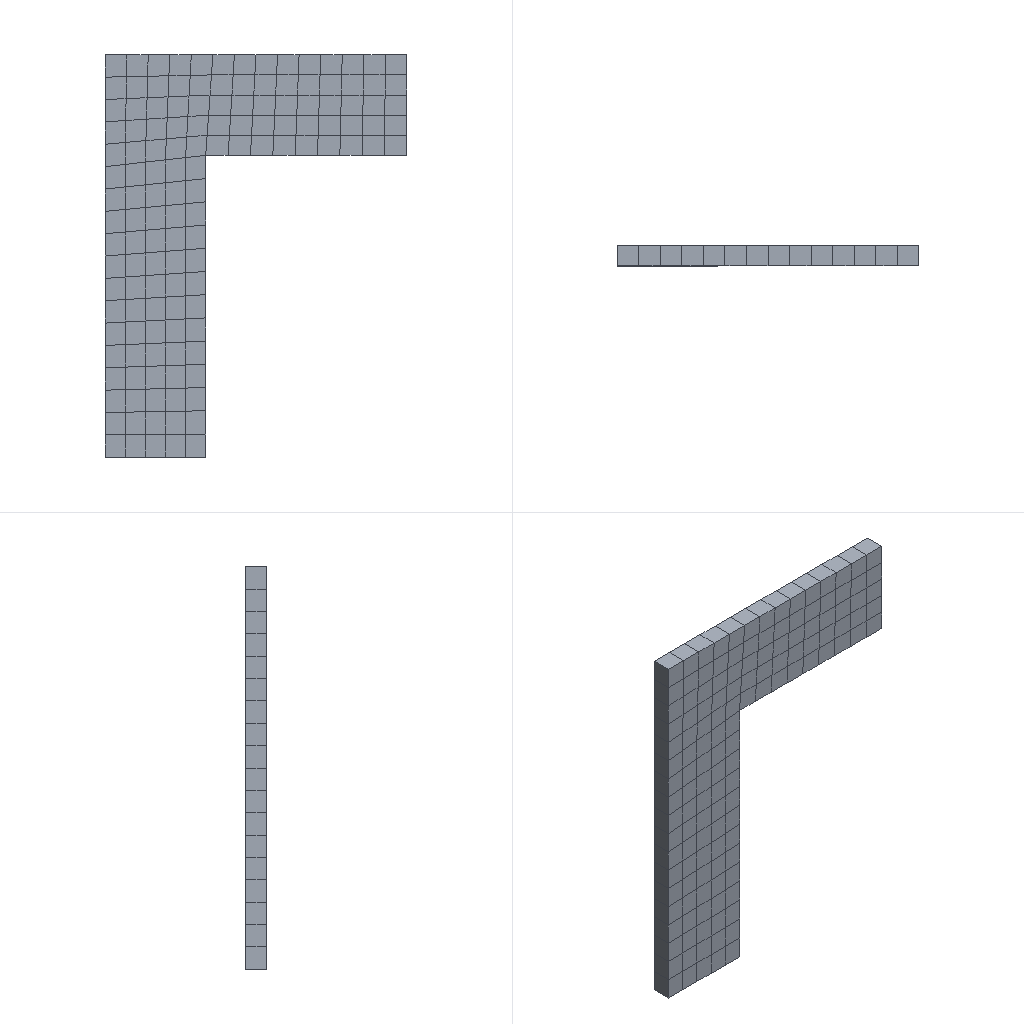Simulation study | ansys workbench
Set-up summary:
category,name,step,type,value,unit,region
solver,ansys_workbench
units,mm-N-s-tonne (MPa),,stated,"/units,MPA"
analysis,LS1,,static
load_step,LS1,LS1,static,nsubst=1; time=1
mesh,nodes,,,1108
mesh,elements,,,140
element_type,SOLID186,,,135
element_type,SURF154,,,5
material,Structural Steel,,E,200000,tonne s^-2 mm^-1
material,Structural Steel,,nu,0.3
material,Structural Steel,,density,7.85e-09,tonne mm^-3
material,Structural Steel,,conductivity,60.5,tonne mm s^-3 C^-1
material,Structural Steel,,specific_heat,4.34e+08,mm^2 s^-2 C^-1
material,Structural Steel,,cte,1.2e-05,C^-1
material,Structural Steel,,permeability,10000
material,Structural Steel,,resistivity,0.00017,ohm mm
load,Define Force Using Surface Effect Elements,LS1,surface-effect pres face 1,-4.65,,SURF154 #2
bc,Fixed Supports,model,fixed,[dofs=ALL],,_FIXEDSU
named_set,_FIXEDSU,,node,93
Ansys APDL input file, long lists of numbers shortened:
/batch
/config,noeldb,1     ! force off writing results to database
*get,_wallstrt,active,,time,wall
! ANSYS input file written by Workbench version 2022 R1
! File used for geometry attach:
/title,wbnew--____ (A5)
! ****** Begin Custom Load Command Snippet ******
/COM, ACT Extensions:
/COM,     LSDYNA, 2021.1
/COM,
! ****** End   Custom Load Command Snippet ******
*DIM,_wb_ProjectScratch_dir,string,248
_wb_ProjectScratch_dir(1) = ''
*DIM,_wb_SolverFiles_dir,string,248
_wb_SolverFiles_dir(1) = ''
*DIM,_wb_userfiles_dir,string,248
_wb_userfiles_dir(1) = ''
/com,--- Data in consistent NMM units. See Solving Units in the help system for more information.
/units,MPA
/nopr
/wb,file,start              !  signify a WB generated input file
/prep7
! Turn off shape checking because checks already performed inside WB mesher.
! See help system for more information.
SHPP,OFF,,NOWARN
/nolist
etcon,set             ! allow ANSYS to choose best KEYOP's for 180x elements, resets any applicable keyopt to MAPDL defaults
/com,*********** Nodes for the whole assembly ***********
nblock,3,,1218
(1i9,3e20.9e3)
        1     3.000000000E+00     0.000000000E+00     9.777777778E+00
! (1107 more lines like these left out)
-1
/wb,elem,start            !  set before creation of elements
/com,*********** Elements for Body 1 "__1-FreeParts|____-____1" ***********
et,1,186
keyo,1,2,1          ! set full integration on SOLID186
eblock,19,solid,,135
(19i9)
        1        1        1        1        0        0        0        0       20        0        1      104      290      291      292      105      255      254      253
! (269 more lines like these left out)
-1
/wb,elem,end               !  done creating elements
/com,*********** Send User Defined Coordinate System(s) ***********
csys,0
toffst,273.15,  ! Temperature offset from absolute zero
/com,*********** Set Reference Temperature ***********
tref,22.
/wb,mat,start              !  starting to send materials
/com,*********** Send Materials ***********
Temperature = 'TEMP' ! Temperature
MP,DENS,1,7.85e-09,	! tonne mm^-3
MP,ALPX,1,1.2e-05,	! C^-1
MP,C,1,434000000,	! mm^2 s^-2 C^-1
MP,KXX,1,60.5,	! tonne mm s^-3 C^-1
MP,RSVX,1,0.00017,	! ohm mm
MP,EX,1,200000,	! tonne s^-2 mm^-1
MP,NUXY,1,0.3,
MP,MURX,1,10000,
/wb,mat,end                !  done sending materials
!************************* Model Summary ********************
!__1-FreeParts|____-____1,	结构钢,	matid,	1
!************************* End Model Summary ********************
! get the diagonal of the bounding box. Needed later for other things
*get,_xmin,node,,mnloc,x
*get,_ymin,node,,mnloc,y
*get,_zmin,node,,mnloc,z
*get,_xmax,node,,mxloc,x
*get,_ymax,node,,mxloc,y
*get,_zmax,node,,mxloc,z
_ASMDIAG=(_xmax-_xmin)*(_xmax-_xmin)+(_ymax-_ymin)*(_ymax-_ymin)+(_zmax-_zmin)*(_zmax-_zmin)
_ASMDIAG=SQRT(_ASMDIAG)
/wb,contact,start          !  starting to send contact
/wb,contact,end            !  done creating contacts
/golist
/wb,load,start             !  starting to send loads
/com,*********** Fixed Supports ***********
CMBLOCK,_FIXEDSU,NODE,       93
(8i10)
       236       237       238       239       240       241       242       243
! (11 more lines like these left out)
cmsel,s,_FIXEDSU
d,all,all
nsel,all
/com,*********** Define Force Using Surface Effect Elements ***********
local,12,0,0.,0.,0.,0.,0.,0.
csys,0
et,2,154
eblock,10,,,5
(15i9)
      470        2        2        2       12      217      218      327      328      934      937     1100      935
      471        2        2        2       12      218      219      326      327      936      939     1099      937
      472        2        2        2       12      219      220      325      326      938      941     1098      939
      473        2        2        2       12      220      221      324      325      940      943     1097      941
      474        2        2        2       12      221      222      323      324      942      945     1096      943
-1
esel,s,type,,2
keyop,2,2,1                ! Apply load in local coordinate system
keyop,2,7,1                ! Use original area so load is constant in large deformation
esel,all
/gst,on,on
fini
*get,_numnode,node,0,count
*get,_numelem,elem,0,count
*get, _MAXELEMNUM, elem, 0, NUM, MAX
*get, _MAXNODENUM, node, 0, NUM, MAX
*get, _MAXELEMTYPE, etyp, 0, NUM, MAX
*get, _MAXREALCONST, real, 0, NUM, MAX
/go
/wb,load,end               !  done creating loads
/com,--- Number of total nodes = %_numnode%
/com,--- Number of contact elements = 5
/com,--- Number of spring elements = 0
/com,--- Number of bearing elements = 0
/com,--- Number of solid elements = 135
/com,--- Number of condensed parts = 0
/com,--- Number of total elements = %_numelem%
*get,_wallbsol,active,,time,wall
/com,****************************************************************************
/com,*************************    SOLUTION       ********************************
/com,****************************************************************************
/solu
antype,0                   ! static analysis
_thickRatio=  0     ! Ratio of thick parts in the model
eqsl,sparse,,,,,1
cntr,print,1               ! print out contact info and also make no initial contact an error
dmpoption,emat,no             ! Don't combine emat file for DANSYS
dmpoption,esav,no             ! Don't combine esav file for DANSYS
nldiag,cont,iter           ! print out contact info each equilibrium iteration
rescontrol,,none                 ! Do not keep any restart files
/com,****************************************************
/com,******************* SOLVE FOR LS 1 OF 1 ****************
esel,s,type,,2
nsle
sfe,all,1,pres,1,-4.65
sfe,all,2,pres,1,0.
sfe,all,3,pres,1,0.
nsel,all
esel,all
/nopr
/gopr
nsub,1,1,1
time,1.
outres,erase
outres,all,none
outres,nsol,all,
outres,rsol,all
outres,eangl,all
outres,etmp,all
outres,veng,all
outres,strs,all,
outres,epel,all,
outres,eppl,all,
outres,cont,all,
! *********** WB SOLVE COMMAND ***********
! check interactive state
*get,ANSINTER_,active,,int
*if,ANSINTER_,ne,0,then
/eof
*endif
solve
/com *************** Write FE CONNECTORS *********
CEWRITE,file,ce,,INTE
/com,****************************************************
/com,*************** FINISHED SOLVE FOR LS 1 *************
*get,_wallasol,active,,time,wall
/nopr
*get,_numnode,node,0,count
*get,_numelem,elem,0,count
*get, _MAXELEMNUM, elem, 0, NUM, MAX
*get, _MAXNODENUM, node, 0, NUM, MAX,,,INTERNAL
*get, _MAXELEMTYPE, etyp, 0, NUM, MAX
*get, _MAXREALCONST, real, 0, NUM, MAX
/gopr
/post1
xmlo,ENCODING,ISO-8859-1
xmlo,parm
/xml,parm,xml
fini
/gopr
*get,_walldone,active,,time,wall
_preptime=(_wallbsol-_wallstrt)*3600
_solvtime=(_wallasol-_wallbsol)*3600
_posttime=(_walldone-_wallasol)*3600
_totaltim=(_walldone-_wallstrt)*3600
*get,_dlbratio,active,0,solu,dlbr
*get,_combtime,active,0,solu,comb
*get,_ssmode,active,0,solu,ssmm
*get,_ndofs,active,0,solu,ndof
*get,_sol_end_time,active,0,set,time
*if,_sol_end_time,eq,1.,then
/fclean				!clean distributed files
*endif
/com,--- Total number of nodes = %_numnode%
/com,--- Total number of elements = %_numelem%
/com,--- Element load balance ratio = %_dlbratio%
/com,--- Time to combine distributed files = %_combtime%
/com,--- Sparse memory mode = %_ssmode%
/com,--- Number of DOF = %_ndofs%
/wb,file,end               ! done with WB generated input
Results summary:
result,analyses[0].index,,,1
result,analyses[0].system,,,SYS
result,analyses[0].deck,,,deck.dat
result,analyses[0].solve_status,,,completed
result,analyses[0].analysis_type,,,static
result,analyses[0].physics,,,mechanical
result,analyses[0].unit_system,,,"NMM: mm, ton, N, s, mV, mA, degC"
result,analyses[0].n_sets,,,1
result,analyses[0].load_steps[0].set,set=1,,1
result,analyses[0].load_steps[0].time_or_freq,set=1,,1
result,analyses[0].load_steps[0].max_displacement_magnitude,set=1,,0.0008504
result,analyses[0].load_steps[0].max_von_mises_nodal,set=1,,6.715
result,analyses[0].load_steps[0].reaction_force_sum_xyz[1],set=1,,93
result,analyses[0].load_steps[0].reaction_force_sum_xyz[2],set=1,,-1.79969e-11
result,analyses[0].load_steps[0].reaction_force_sum_xyz[3],set=1,,8.03191e-13